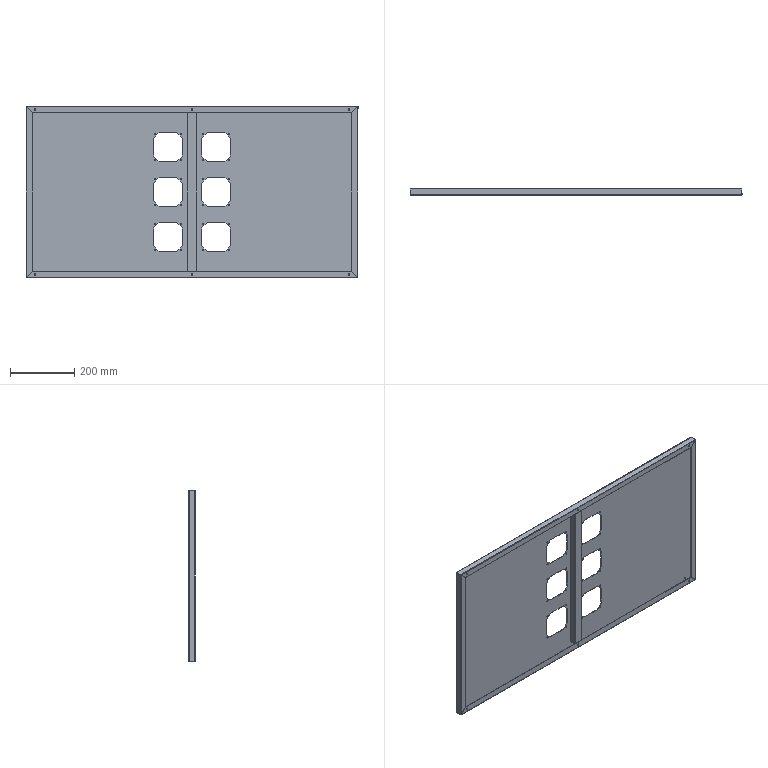Part | SolidWorks | 2 solids | 212 faces | box 1035 x 20 x 535 mm | volume 656761 mm3 | cylinder 116 | plane 80 | spline 16 | commonest cylinder face diameters 4.5 x72 105 x24 0.2 x10 2.2 x10